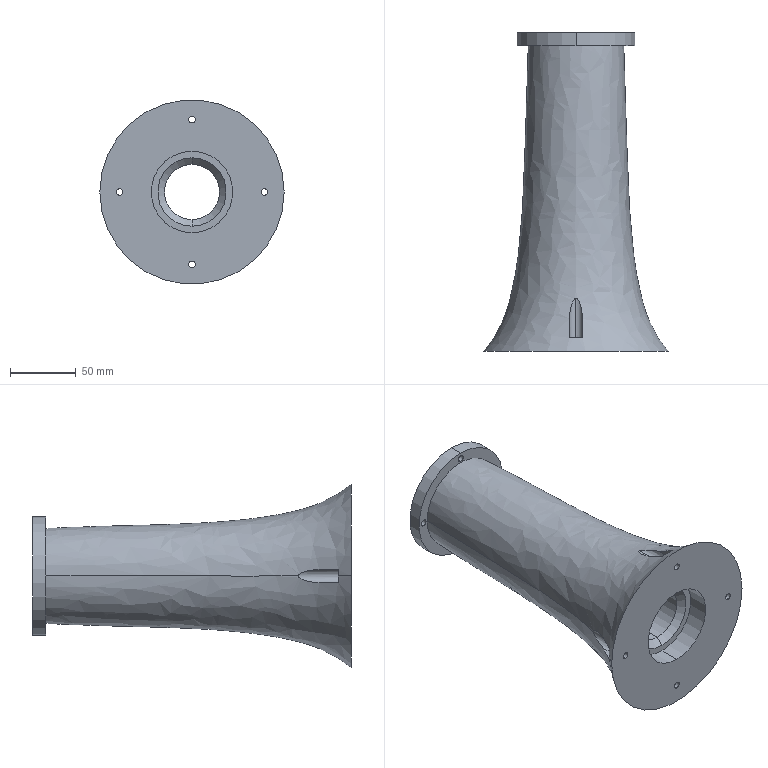Part | NX | features BREP 1 | 1 solid | 52 faces | box 140 x 242 x 140 mm | volume 1087762 mm3 | cylinder 29 | plane 17 | cone 4 | spline 2 | commonest cylinder face diameters 5 x8 5.2 x8 10 x5 62 x4 42 x2 90 x2